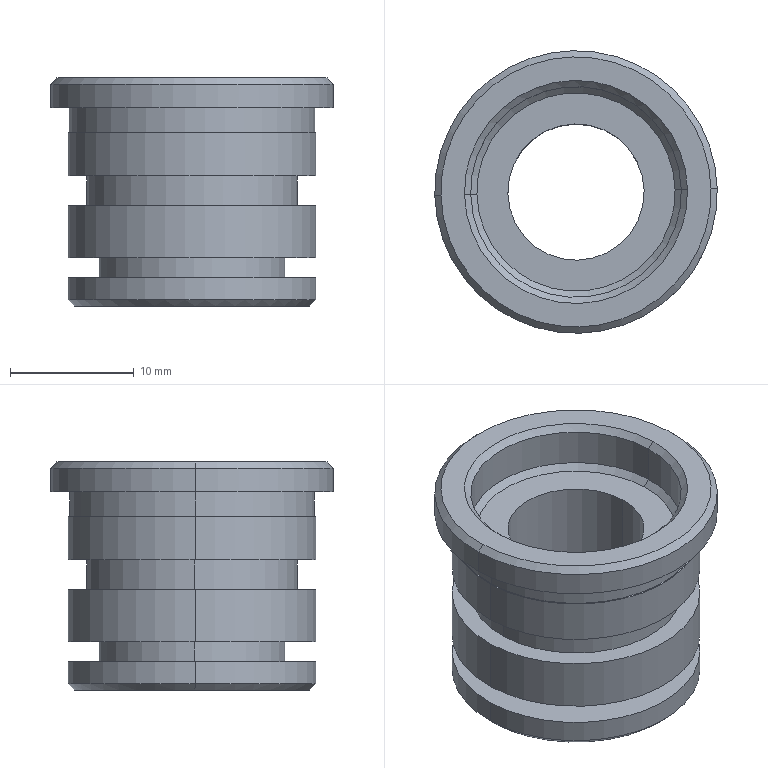Part | SolidWorks | features BaseBody 1 | 1 solid | 37 faces | box 22.8 x 22.8 x 18.4 mm | volume 3267 mm3 | cylinder 18 | cone 10 | plane 9 | commonest cylinder face diameters 20 x6 17 x4 11 x2 15 x2 19.8 x2 22.8 x2
STEP:
#1=CARTESIAN_POINT('',(394.496,102.788,49.));
#2=VERTEX_POINT('',#1);
#3=CARTESIAN_POINT('',(371.704,102.212,49.));
#4=VERTEX_POINT('',#3);
#5=CARTESIAN_POINT('',(383.1,102.5,49.));
#6=DIRECTION('',(0.,0.,-1.));
#7=DIRECTION('',(0.9997,0.02523,0.));
#8=AXIS2_PLACEMENT_3D('',#5,#6,#7);
#9=CIRCLE('',#8,11.4);
#10=EDGE_CURVE('',#2,#4,#9,.T.);
#11=ORIENTED_EDGE('',*,*,#10,.T.);
#12=CARTESIAN_POINT('',(371.704,102.212,47.1));
#13=VERTEX_POINT('',#12);
#14=CARTESIAN_POINT('',(371.704,102.212,25.779));
#15=DIRECTION('',(0.,0.,-1.));
#16=VECTOR('',#15,1000.);
#17=LINE('',#14,#16);
#18=EDGE_CURVE('',#4,#13,#17,.T.);
#19=ORIENTED_EDGE('',*,*,#18,.T.);
#20=CARTESIAN_POINT('',(394.496,102.788,47.1));
#21=VERTEX_POINT('',#20);
#22=CARTESIAN_POINT('',(383.1,102.5,47.1));
#23=DIRECTION('',(0.,0.,-1.));
#24=DIRECTION('',(0.9997,0.02523,0.));
#25=AXIS2_PLACEMENT_3D('',#22,#23,#24);
#26=CIRCLE('',#25,11.4);
#27=EDGE_CURVE('',#21,#13,#26,.T.);
#28=ORIENTED_EDGE('',*,*,#27,.F.);
#29=CARTESIAN_POINT('',(394.496,102.788,25.779));
#30=DIRECTION('',(0.,0.,-1.));
#31=VECTOR('',#30,1000.);
#32=LINE('',#29,#31);
#33=EDGE_CURVE('',#2,#21,#32,.T.);
#34=ORIENTED_EDGE('',*,*,#33,.F.);
#35=EDGE_LOOP('',(#11,#19,#28,#34));
#36=FACE_OUTER_BOUND('',#35,.T.);
#37=CARTESIAN_POINT('',(383.1,102.5,25.779));
#38=DIRECTION('',(0.,0.,-1.));
#39=DIRECTION('',(0.9997,0.02523,0.));
#40=AXIS2_PLACEMENT_3D('',#37,#38,#39);
#41=CYLINDRICAL_SURFACE('',#40,11.4);
#42=ADVANCED_FACE('',(#36),#41,.T.);
#43=CARTESIAN_POINT('',(393.997,102.775,49.5));
#44=VERTEX_POINT('',#43);
#45=CARTESIAN_POINT('',(372.203,102.225,49.5));
#46=VERTEX_POINT('',#45);
#47=CARTESIAN_POINT('',(383.1,102.5,49.5));
#48=DIRECTION('',(0.,0.,-1.));
#49=DIRECTION('',(0.9997,0.02523,0.));
#50=AXIS2_PLACEMENT_3D('',#47,#48,#49);
#51=CIRCLE('',#50,10.9);
#52=EDGE_CURVE('',#44,#46,#51,.T.);
#53=ORIENTED_EDGE('',*,*,#52,.T.);
#54=CARTESIAN_POINT('',(371.704,102.212,49.));
#55=DIRECTION('',(-0.7069,-0.01784,-0.7071));
#56=VECTOR('',#55,1000.);
#57=LINE('',#54,#56);
#58=EDGE_CURVE('',#46,#4,#57,.T.);
#59=ORIENTED_EDGE('',*,*,#58,.T.);
#60=ORIENTED_EDGE('',*,*,#10,.F.);
#61=CARTESIAN_POINT('',(394.496,102.788,49.));
#62=DIRECTION('',(0.7069,0.01784,-0.7071));
#63=VECTOR('',#62,1000.);
#64=LINE('',#61,#63);
#65=EDGE_CURVE('',#44,#2,#64,.T.);
#66=ORIENTED_EDGE('',*,*,#65,.F.);
#67=EDGE_LOOP('',(#53,#59,#60,#66));
#68=FACE_OUTER_BOUND('',#67,.T.);
#69=CARTESIAN_POINT('',(383.1,102.5,49.));
#70=DIRECTION('',(0.,0.,-1.));
#71=DIRECTION('',(0.9997,0.02523,0.));
#72=AXIS2_PLACEMENT_3D('',#69,#70,#71);
#73=CONICAL_SURFACE('',#72,11.4,0.7854);
#74=ADVANCED_FACE('',(#68),#73,.T.);
#75=CARTESIAN_POINT('',(374.603,102.286,49.));
#76=VERTEX_POINT('',#75);
#77=CARTESIAN_POINT('',(391.597,102.714,49.));
#78=VERTEX_POINT('',#77);
#79=CARTESIAN_POINT('',(383.1,102.5,49.));
#80=DIRECTION('',(0.,0.,-1.));
#81=DIRECTION('',(0.9997,0.02523,0.));
#82=AXIS2_PLACEMENT_3D('',#79,#80,#81);
#83=CIRCLE('',#82,8.5);
#84=EDGE_CURVE('',#76,#78,#83,.T.);
#85=ORIENTED_EDGE('',*,*,#84,.T.);
#86=CARTESIAN_POINT('',(392.097,102.727,49.5));
#87=VERTEX_POINT('',#86);
#88=CARTESIAN_POINT('',(392.097,102.727,49.5));
#89=DIRECTION('',(0.7069,0.01784,0.7071));
#90=VECTOR('',#89,1000.);
#91=LINE('',#88,#90);
#92=EDGE_CURVE('',#78,#87,#91,.T.);
#93=ORIENTED_EDGE('',*,*,#92,.T.);
#94=CARTESIAN_POINT('',(374.103,102.273,49.5));
#95=VERTEX_POINT('',#94);
#96=CARTESIAN_POINT('',(383.1,102.5,49.5));
#97=DIRECTION('',(0.,0.,-1.));
#98=DIRECTION('',(0.9997,0.02523,0.));
#99=AXIS2_PLACEMENT_3D('',#96,#97,#98);
#100=CIRCLE('',#99,9.);
#101=EDGE_CURVE('',#95,#87,#100,.T.);
#102=ORIENTED_EDGE('',*,*,#101,.F.);
#103=CARTESIAN_POINT('',(374.103,102.273,49.5));
#104=DIRECTION('',(-0.7069,-0.01784,0.7071));
#105=VECTOR('',#104,1000.);
#106=LINE('',#103,#105);
#107=EDGE_CURVE('',#76,#95,#106,.T.);
#108=ORIENTED_EDGE('',*,*,#107,.F.);
#109=EDGE_LOOP('',(#85,#93,#102,#108));
#110=FACE_OUTER_BOUND('',#109,.T.);
#111=CARTESIAN_POINT('',(383.1,102.5,49.5));
#112=DIRECTION('',(0.,0.,1.));
#113=DIRECTION('',(-0.9997,-0.02523,0.));
#114=AXIS2_PLACEMENT_3D('',#111,#112,#113);
#115=CONICAL_SURFACE('',#114,9.,0.7854);
#116=ADVANCED_FACE('',(#110),#115,.F.);
#117=ORIENTED_EDGE('',*,*,#84,.F.);
#118=CARTESIAN_POINT('',(374.603,102.286,46.));
#119=VERTEX_POINT('',#118);
#120=CARTESIAN_POINT('',(374.603,102.286,25.779));
#121=DIRECTION('',(0.,0.,-1.));
#122=VECTOR('',#121,1000.);
#123=LINE('',#120,#122);
#124=EDGE_CURVE('',#76,#119,#123,.T.);
#125=ORIENTED_EDGE('',*,*,#124,.T.);
#126=CARTESIAN_POINT('',(391.597,102.714,46.));
#127=VERTEX_POINT('',#126);
#128=CARTESIAN_POINT('',(383.1,102.5,46.));
#129=DIRECTION('',(0.,0.,-1.));
#130=DIRECTION('',(0.9997,0.02523,0.));
#131=AXIS2_PLACEMENT_3D('',#128,#129,#130);
#132=CIRCLE('',#131,8.5);
#133=EDGE_CURVE('',#119,#127,#132,.T.);
#134=ORIENTED_EDGE('',*,*,#133,.T.);
#135=CARTESIAN_POINT('',(391.597,102.714,25.779));
#136=DIRECTION('',(0.,0.,-1.));
#137=VECTOR('',#136,1000.);
#138=LINE('',#135,#137);
#139=EDGE_CURVE('',#78,#127,#138,.T.);
#140=ORIENTED_EDGE('',*,*,#139,.F.);
#141=EDGE_LOOP('',(#117,#125,#134,#140));
#142=FACE_OUTER_BOUND('',#141,.T.);
#143=CARTESIAN_POINT('',(383.1,102.5,25.779));
#144=DIRECTION('',(0.,0.,-1.));
#145=DIRECTION('',(0.9997,0.02523,0.));
#146=AXIS2_PLACEMENT_3D('',#143,#144,#145);
#147=CYLINDRICAL_SURFACE('',#146,8.5);
#148=ADVANCED_FACE('',(#142),#147,.F.);
#149=CARTESIAN_POINT('',(375.103,102.298,45.5));
#150=VERTEX_POINT('',#149);
#151=CARTESIAN_POINT('',(391.097,102.702,45.5));
#152=VERTEX_POINT('',#151);
#153=CARTESIAN_POINT('',(383.1,102.5,45.5));
#154=DIRECTION('',(0.,0.,-1.));
#155=DIRECTION('',(0.9997,0.02523,0.));
#156=AXIS2_PLACEMENT_3D('',#153,#154,#155);
#157=CIRCLE('',#156,8.);
#158=EDGE_CURVE('',#150,#152,#157,.T.);
#159=ORIENTED_EDGE('',*,*,#158,.T.);
#160=CARTESIAN_POINT('',(391.597,102.714,46.));
#161=DIRECTION('',(0.7069,0.01784,0.7071));
#162=VECTOR('',#161,1000.);
#163=LINE('',#160,#162);
#164=EDGE_CURVE('',#152,#127,#163,.T.);
#165=ORIENTED_EDGE('',*,*,#164,.T.);
#166=ORIENTED_EDGE('',*,*,#133,.F.);
#167=CARTESIAN_POINT('',(374.603,102.286,46.));
#168=DIRECTION('',(-0.7069,-0.01784,0.7071));
#169=VECTOR('',#168,1000.);
#170=LINE('',#167,#169);
#171=EDGE_CURVE('',#150,#119,#170,.T.);
#172=ORIENTED_EDGE('',*,*,#171,.F.);
#173=EDGE_LOOP('',(#159,#165,#166,#172));
#174=FACE_OUTER_BOUND('',#173,.T.);
#175=CARTESIAN_POINT('',(383.1,102.5,46.));
#176=DIRECTION('',(0.,0.,1.));
#177=DIRECTION('',(-0.9997,-0.02523,0.));
#178=AXIS2_PLACEMENT_3D('',#175,#176,#177);
#179=CONICAL_SURFACE('',#178,8.5,0.7854);
#180=ADVANCED_FACE('',(#174),#179,.F.);
#181=CARTESIAN_POINT('',(377.602,102.361,45.5));
#182=VERTEX_POINT('',#181);
#183=CARTESIAN_POINT('',(388.598,102.639,45.5));
#184=VERTEX_POINT('',#183);
#185=CARTESIAN_POINT('',(383.1,102.5,45.5));
#186=DIRECTION('',(0.,0.,-1.));
#187=DIRECTION('',(0.9997,0.02523,0.));
#188=AXIS2_PLACEMENT_3D('',#185,#186,#187);
#189=CIRCLE('',#188,5.5);
#190=EDGE_CURVE('',#182,#184,#189,.T.);
#191=ORIENTED_EDGE('',*,*,#190,.F.);
#192=CARTESIAN_POINT('',(377.602,102.361,31.6));
#193=VERTEX_POINT('',#192);
#194=CARTESIAN_POINT('',(377.602,102.361,25.779));
#195=DIRECTION('',(0.,0.,-1.));
#196=VECTOR('',#195,1000.);
#197=LINE('',#194,#196);
#198=EDGE_CURVE('',#182,#193,#197,.T.);
#199=ORIENTED_EDGE('',*,*,#198,.T.);
#200=CARTESIAN_POINT('',(388.598,102.639,31.6));
#201=VERTEX_POINT('',#200);
#202=CARTESIAN_POINT('',(383.1,102.5,31.6));
#203=DIRECTION('',(0.,0.,-1.));
#204=DIRECTION('',(0.9997,0.02523,0.));
#205=AXIS2_PLACEMENT_3D('',#202,#203,#204);
#206=CIRCLE('',#205,5.5);
#207=EDGE_CURVE('',#193,#201,#206,.T.);
#208=ORIENTED_EDGE('',*,*,#207,.T.);
#209=CARTESIAN_POINT('',(388.598,102.639,25.779));
#210=DIRECTION('',(0.,0.,-1.));
#211=VECTOR('',#210,1000.);
#212=LINE('',#209,#211);
#213=EDGE_CURVE('',#184,#201,#212,.T.);
#214=ORIENTED_EDGE('',*,*,#213,.F.);
#215=EDGE_LOOP('',(#191,#199,#208,#214));
#216=FACE_OUTER_BOUND('',#215,.T.);
#217=CARTESIAN_POINT('',(383.1,102.5,25.779));
#218=DIRECTION('',(0.,0.,-1.));
#219=DIRECTION('',(0.9997,0.02523,0.));
#220=AXIS2_PLACEMENT_3D('',#217,#218,#219);
#221=CYLINDRICAL_SURFACE('',#220,5.5);
#222=ADVANCED_FACE('',(#216),#221,.F.);
#223=ORIENTED_EDGE('',*,*,#207,.F.);
#224=CARTESIAN_POINT('',(377.102,102.349,31.1));
#225=VERTEX_POINT('',#224);
#226=CARTESIAN_POINT('',(377.602,102.361,31.6));
#227=DIRECTION('',(-0.7069,-0.01784,-0.7071));
#228=VECTOR('',#227,1000.);
#229=LINE('',#226,#228);
#230=EDGE_CURVE('',#193,#225,#229,.T.);
#231=ORIENTED_EDGE('',*,*,#230,.T.);
#232=CARTESIAN_POINT('',(389.098,102.651,31.1));
#233=VERTEX_POINT('',#232);
#234=CARTESIAN_POINT('',(383.1,102.5,31.1));
#235=DIRECTION('',(0.,0.,-1.));
#236=DIRECTION('',(0.9997,0.02523,0.));
#237=AXIS2_PLACEMENT_3D('',#234,#235,#236);
#238=CIRCLE('',#237,6.);
#239=EDGE_CURVE('',#225,#233,#238,.T.);
#240=ORIENTED_EDGE('',*,*,#239,.T.);
#241=CARTESIAN_POINT('',(388.598,102.639,31.6));
#242=DIRECTION('',(0.7069,0.01784,-0.7071));
#243=VECTOR('',#242,1000.);
#244=LINE('',#241,#243);
#245=EDGE_CURVE('',#201,#233,#244,.T.);
#246=ORIENTED_EDGE('',*,*,#245,.F.);
#247=EDGE_LOOP('',(#223,#231,#240,#246));
#248=FACE_OUTER_BOUND('',#247,.T.);
#249=CARTESIAN_POINT('',(383.1,102.5,31.6));
#250=DIRECTION('',(0.,0.,-1.));
#251=DIRECTION('',(0.9997,0.02523,0.));
#252=AXIS2_PLACEMENT_3D('',#249,#250,#251);
#253=CONICAL_SURFACE('',#252,5.5,0.7854);
#254=ADVANCED_FACE('',(#248),#253,.F.);
#255=CARTESIAN_POINT('',(392.597,102.74,31.1));
#256=VERTEX_POINT('',#255);
#257=CARTESIAN_POINT('',(373.603,102.26,31.1));
#258=VERTEX_POINT('',#257);
#259=CARTESIAN_POINT('',(383.1,102.5,31.1));
#260=DIRECTION('',(0.,0.,-1.));
#261=DIRECTION('',(0.9997,0.02523,0.));
#262=AXIS2_PLACEMENT_3D('',#259,#260,#261);
#263=CIRCLE('',#262,9.5);
#264=EDGE_CURVE('',#256,#258,#263,.T.);
#265=ORIENTED_EDGE('',*,*,#264,.F.);
#266=CARTESIAN_POINT('',(393.097,102.752,31.6));
#267=VERTEX_POINT('',#266);
#268=CARTESIAN_POINT('',(392.597,102.74,31.1));
#269=DIRECTION('',(0.7069,0.01784,0.7071));
#270=VECTOR('',#269,1000.);
#271=LINE('',#268,#270);
#272=EDGE_CURVE('',#256,#267,#271,.T.);
#273=ORIENTED_EDGE('',*,*,#272,.T.);
#274=CARTESIAN_POINT('',(373.103,102.248,31.6));
#275=VERTEX_POINT('',#274);
#276=CARTESIAN_POINT('',(383.1,102.5,31.6));
#277=DIRECTION('',(0.,0.,-1.));
#278=DIRECTION('',(0.9997,0.02523,0.));
#279=AXIS2_PLACEMENT_3D('',#276,#277,#278);
#280=CIRCLE('',#279,10.);
#281=EDGE_CURVE('',#267,#275,#280,.T.);
#282=ORIENTED_EDGE('',*,*,#281,.T.);
#283=CARTESIAN_POINT('',(373.603,102.26,31.1));
#284=DIRECTION('',(-0.7069,-0.01784,0.7071));
#285=VECTOR('',#284,1000.);
#286=LINE('',#283,#285);
#287=EDGE_CURVE('',#258,#275,#286,.T.);
#288=ORIENTED_EDGE('',*,*,#287,.F.);
#289=EDGE_LOOP('',(#265,#273,#282,#288));
#290=FACE_OUTER_BOUND('',#289,.T.);
#291=CARTESIAN_POINT('',(383.1,102.5,31.1));
#292=DIRECTION('',(0.,0.,1.));
#293=DIRECTION('',(-0.9997,-0.02523,0.));
#294=AXIS2_PLACEMENT_3D('',#291,#292,#293);
#295=CONICAL_SURFACE('',#294,9.5,0.7854);
#296=ADVANCED_FACE('',(#290),#295,.T.);
#297=CARTESIAN_POINT('',(393.097,102.752,33.4));
#298=VERTEX_POINT('',#297);
#299=CARTESIAN_POINT('',(373.103,102.248,33.4));
#300=VERTEX_POINT('',#299);
#301=CARTESIAN_POINT('',(383.1,102.5,33.4));
#302=DIRECTION('',(0.,0.,-1.));
#303=DIRECTION('',(0.9997,0.02523,0.));
#304=AXIS2_PLACEMENT_3D('',#301,#302,#303);
#305=CIRCLE('',#304,10.);
#306=EDGE_CURVE('',#298,#300,#305,.T.);
#307=ORIENTED_EDGE('',*,*,#306,.T.);
#308=CARTESIAN_POINT('',(373.103,102.248,25.779));
#309=DIRECTION('',(0.,0.,-1.));
#310=VECTOR('',#309,1000.);
#311=LINE('',#308,#310);
#312=EDGE_CURVE('',#300,#275,#311,.T.);
#313=ORIENTED_EDGE('',*,*,#312,.T.);
#314=ORIENTED_EDGE('',*,*,#281,.F.);
#315=CARTESIAN_POINT('',(393.097,102.752,25.779));
#316=DIRECTION('',(0.,0.,-1.));
#317=VECTOR('',#316,1000.);
#318=LINE('',#315,#317);
#319=EDGE_CURVE('',#298,#267,#318,.T.);
#320=ORIENTED_EDGE('',*,*,#319,.F.);
#321=EDGE_LOOP('',(#307,#313,#314,#320));
#322=FACE_OUTER_BOUND('',#321,.T.);
#323=CARTESIAN_POINT('',(383.1,102.5,25.779));
#324=DIRECTION('',(0.,0.,-1.));
#325=DIRECTION('',(0.9997,0.02523,0.));
#326=AXIS2_PLACEMENT_3D('',#323,#324,#325);
#327=CYLINDRICAL_SURFACE('',#326,10.);
#328=ADVANCED_FACE('',(#322),#327,.T.);
#329=CARTESIAN_POINT('',(390.598,102.689,35.));
#330=VERTEX_POINT('',#329);
#331=CARTESIAN_POINT('',(375.602,102.311,35.));
#332=VERTEX_POINT('',#331);
#333=CARTESIAN_POINT('',(383.1,102.5,35.));
#334=DIRECTION('',(0.,0.,-1.));
#335=DIRECTION('',(0.9997,0.02523,0.));
#336=AXIS2_PLACEMENT_3D('',#333,#334,#335);
#337=CIRCLE('',#336,7.5);
#338=EDGE_CURVE('',#330,#332,#337,.T.);
#339=ORIENTED_EDGE('',*,*,#338,.T.);
#340=CARTESIAN_POINT('',(375.602,102.311,33.4));
#341=VERTEX_POINT('',#340);
#342=CARTESIAN_POINT('',(375.602,102.311,25.779));
#343=DIRECTION('',(0.,0.,-1.));
#344=VECTOR('',#343,1000.);
#345=LINE('',#342,#344);
#346=EDGE_CURVE('',#332,#341,#345,.T.);
#347=ORIENTED_EDGE('',*,*,#346,.T.);
#348=CARTESIAN_POINT('',(390.598,102.689,33.4));
#349=VERTEX_POINT('',#348);
#350=CARTESIAN_POINT('',(383.1,102.5,33.4));
#351=DIRECTION('',(0.,0.,-1.));
#352=DIRECTION('',(0.9997,0.02523,0.));
#353=AXIS2_PLACEMENT_3D('',#350,#351,#352);
#354=CIRCLE('',#353,7.5);
#355=EDGE_CURVE('',#349,#341,#354,.T.);
#356=ORIENTED_EDGE('',*,*,#355,.F.);
#357=CARTESIAN_POINT('',(390.598,102.689,25.779));
#358=DIRECTION('',(0.,0.,-1.));
#359=VECTOR('',#358,1000.);
#360=LINE('',#357,#359);
#361=EDGE_CURVE('',#330,#349,#360,.T.);
#362=ORIENTED_EDGE('',*,*,#361,.F.);
#363=EDGE_LOOP('',(#339,#347,#356,#362));
#364=FACE_OUTER_BOUND('',#363,.T.);
#365=CARTESIAN_POINT('',(383.1,102.5,25.779));
#366=DIRECTION('',(0.,0.,-1.));
#367=DIRECTION('',(0.9997,0.02523,0.));
#368=AXIS2_PLACEMENT_3D('',#365,#366,#367);
#369=CYLINDRICAL_SURFACE('',#368,7.5);
#370=ADVANCED_FACE('',(#364),#369,.T.);
#371=CARTESIAN_POINT('',(393.097,102.752,39.2));
#372=VERTEX_POINT('',#371);
#373=CARTESIAN_POINT('',(373.103,102.248,39.2));
#374=VERTEX_POINT('',#373);
#375=CARTESIAN_POINT('',(383.1,102.5,39.2));
#376=DIRECTION('',(0.,0.,-1.));
#377=DIRECTION('',(0.9997,0.02523,0.));
#378=AXIS2_PLACEMENT_3D('',#375,#376,#377);
#379=CIRCLE('',#378,10.);
#380=EDGE_CURVE('',#372,#374,#379,.T.);
#381=ORIENTED_EDGE('',*,*,#380,.T.);
#382=CARTESIAN_POINT('',(373.103,102.248,35.));
#383=VERTEX_POINT('',#382);
#384=CARTESIAN_POINT('',(373.103,102.248,25.779));
#385=DIRECTION('',(0.,0.,-1.));
#386=VECTOR('',#385,1000.);
#387=LINE('',#384,#386);
#388=EDGE_CURVE('',#374,#383,#387,.T.);
#389=ORIENTED_EDGE('',*,*,#388,.T.);
#390=CARTESIAN_POINT('',(393.097,102.752,35.));
#391=VERTEX_POINT('',#390);
#392=CARTESIAN_POINT('',(383.1,102.5,35.));
#393=DIRECTION('',(0.,0.,-1.));
#394=DIRECTION('',(0.9997,0.02523,0.));
#395=AXIS2_PLACEMENT_3D('',#392,#393,#394);
#396=CIRCLE('',#395,10.);
#397=EDGE_CURVE('',#391,#383,#396,.T.);
#398=ORIENTED_EDGE('',*,*,#397,.F.);
#399=CARTESIAN_POINT('',(393.097,102.752,25.779));
#400=DIRECTION('',(0.,0.,-1.));
#401=VECTOR('',#400,1000.);
#402=LINE('',#399,#401);
#403=EDGE_CURVE('',#372,#391,#402,.T.);
#404=ORIENTED_EDGE('',*,*,#403,.F.);
#405=EDGE_LOOP('',(#381,#389,#398,#404));
#406=FACE_OUTER_BOUND('',#405,.T.);
#407=CARTESIAN_POINT('',(383.1,102.5,25.779));
#408=DIRECTION('',(0.,0.,-1.));
#409=DIRECTION('',(0.9997,0.02523,0.));
#410=AXIS2_PLACEMENT_3D('',#407,#408,#409);
#411=CYLINDRICAL_SURFACE('',#410,10.);
#412=ADVANCED_FACE('',(#406),#411,.T.);
#413=CARTESIAN_POINT('',(391.597,102.714,41.6));
#414=VERTEX_POINT('',#413);
#415=CARTESIAN_POINT('',(374.603,102.286,41.6));
#416=VERTEX_POINT('',#415);
#417=CARTESIAN_POINT('',(383.1,102.5,41.6));
#418=DIRECTION('',(0.,0.,-1.));
#419=DIRECTION('',(0.9997,0.02523,0.));
#420=AXIS2_PLACEMENT_3D('',#417,#418,#419);
#421=CIRCLE('',#420,8.5);
#422=EDGE_CURVE('',#414,#416,#421,.T.);
#423=ORIENTED_EDGE('',*,*,#422,.T.);
#424=CARTESIAN_POINT('',(374.603,102.286,39.2));
#425=VERTEX_POINT('',#424);
#426=CARTESIAN_POINT('',(374.603,102.286,25.779));
#427=DIRECTION('',(0.,0.,-1.));
#428=VECTOR('',#427,1000.);
#429=LINE('',#426,#428);
#430=EDGE_CURVE('',#416,#425,#429,.T.);
#431=ORIENTED_EDGE('',*,*,#430,.T.);
#432=CARTESIAN_POINT('',(391.597,102.714,39.2));
#433=VERTEX_POINT('',#432);
#434=CARTESIAN_POINT('',(383.1,102.5,39.2));
#435=DIRECTION('',(0.,0.,-1.));
#436=DIRECTION('',(0.9997,0.02523,0.));
#437=AXIS2_PLACEMENT_3D('',#434,#435,#436);
#438=CIRCLE('',#437,8.5);
#439=EDGE_CURVE('',#433,#425,#438,.T.);
#440=ORIENTED_EDGE('',*,*,#439,.F.);
#441=CARTESIAN_POINT('',(391.597,102.714,25.779));
#442=DIRECTION('',(0.,0.,-1.));
#443=VECTOR('',#442,1000.);
#444=LINE('',#441,#443);
#445=EDGE_CURVE('',#414,#433,#444,.T.);
#446=ORIENTED_EDGE('',*,*,#445,.F.);
#447=EDGE_LOOP('',(#423,#431,#440,#446));
#448=FACE_OUTER_BOUND('',#447,.T.);
#449=CARTESIAN_POINT('',(383.1,102.5,25.779));
#450=DIRECTION('',(0.,0.,-1.));
#451=DIRECTION('',(0.9997,0.02523,0.));
#452=AXIS2_PLACEMENT_3D('',#449,#450,#451);
#453=CYLINDRICAL_SURFACE('',#452,8.5);
#454=ADVANCED_FACE('',(#448),#453,.T.);
#455=CARTESIAN_POINT('',(393.097,102.752,45.1));
#456=VERTEX_POINT('',#455);
#457=CARTESIAN_POINT('',(373.103,102.248,45.1));
#458=VERTEX_POINT('',#457);
#459=CARTESIAN_POINT('',(383.1,102.5,45.1));
#460=DIRECTION('',(0.,0.,-1.));
#461=DIRECTION('',(0.9997,0.02523,0.));
#462=AXIS2_PLACEMENT_3D('',#459,#460,#461);
#463=CIRCLE('',#462,10.);
#464=EDGE_CURVE('',#456,#458,#463,.T.);
#465=ORIENTED_EDGE('',*,*,#464,.T.);
#466=CARTESIAN_POINT('',(373.103,102.248,41.6));
#467=VERTEX_POINT('',#466);
#468=CARTESIAN_POINT('',(373.103,102.248,25.779));
#469=DIRECTION('',(0.,0.,-1.));
#470=VECTOR('',#469,1000.);
#471=LINE('',#468,#470);
#472=EDGE_CURVE('',#458,#467,#471,.T.);
#473=ORIENTED_EDGE('',*,*,#472,.T.);
#474=CARTESIAN_POINT('',(393.097,102.752,41.6));
#475=VERTEX_POINT('',#474);
#476=CARTESIAN_POINT('',(383.1,102.5,41.6));
#477=DIRECTION('',(0.,0.,-1.));
#478=DIRECTION('',(0.9997,0.02523,0.));
#479=AXIS2_PLACEMENT_3D('',#476,#477,#478);
#480=CIRCLE('',#479,10.);
#481=EDGE_CURVE('',#475,#467,#480,.T.);
#482=ORIENTED_EDGE('',*,*,#481,.F.);
#483=CARTESIAN_POINT('',(393.097,102.752,25.779));
#484=DIRECTION('',(0.,0.,-1.));
#485=VECTOR('',#484,1000.);
#486=LINE('',#483,#485);
#487=EDGE_CURVE('',#456,#475,#486,.T.);
#488=ORIENTED_EDGE('',*,*,#487,.F.);
#489=EDGE_LOOP('',(#465,#473,#482,#488));
#490=FACE_OUTER_BOUND('',#489,.T.);
#491=CARTESIAN_POINT('',(383.1,102.5,25.779));
#492=DIRECTION('',(0.,0.,-1.));
#493=DIRECTION('',(0.9997,0.02523,0.));
#494=AXIS2_PLACEMENT_3D('',#491,#492,#493);
#495=CYLINDRICAL_SURFACE('',#494,10.);
#496=ADVANCED_FACE('',(#490),#495,.T.);
#497=CARTESIAN_POINT('',(392.997,102.75,47.1));
#498=VERTEX_POINT('',#497);
#499=CARTESIAN_POINT('',(373.203,102.25,47.1));
#500=VERTEX_POINT('',#499);
#501=CARTESIAN_POINT('',(383.1,102.5,47.1));
#502=DIRECTION('',(0.,0.,-1.));
#503=DIRECTION('',(0.9997,0.02523,0.));
#504=AXIS2_PLACEMENT_3D('',#501,#502,#503);
#505=CIRCLE('',#504,9.9);
#506=EDGE_CURVE('',#498,#500,#505,.T.);
#507=ORIENTED_EDGE('',*,*,#506,.T.);
#508=CARTESIAN_POINT('',(373.203,102.25,45.1));
#509=VERTEX_POINT('',#508);
#510=CARTESIAN_POINT('',(373.203,102.25,25.779));
#511=DIRECTION('',(0.,0.,-1.));
#512=VECTOR('',#511,1000.);
#513=LINE('',#510,#512);
#514=EDGE_CURVE('',#500,#509,#513,.T.);
#515=ORIENTED_EDGE('',*,*,#514,.T.);
#516=CARTESIAN_POINT('',(392.997,102.75,45.1));
#517=VERTEX_POINT('',#516);
#518=CARTESIAN_POINT('',(383.1,102.5,45.1));
#519=DIRECTION('',(0.,0.,-1.));
#520=DIRECTION('',(0.9997,0.02523,0.));
#521=AXIS2_PLACEMENT_3D('',#518,#519,#520);
#522=CIRCLE('',#521,9.9);
#523=EDGE_CURVE('',#517,#509,#522,.T.);
#524=ORIENTED_EDGE('',*,*,#523,.F.);
#525=CARTESIAN_POINT('',(392.997,102.75,25.779));
#526=DIRECTION('',(0.,0.,-1.));
#527=VECTOR('',#526,1000.);
#528=LINE('',#525,#527);
#529=EDGE_CURVE('',#498,#517,#528,.T.);
#530=ORIENTED_EDGE('',*,*,#529,.F.);
#531=EDGE_LOOP('',(#507,#515,#524,#530));
#532=FACE_OUTER_BOUND('',#531,.T.);
#533=CARTESIAN_POINT('',(383.1,102.5,25.779));
#534=DIRECTION('',(0.,0.,-1.));
#535=DIRECTION('',(0.9997,0.02523,0.));
#536=AXIS2_PLACEMENT_3D('',#533,#534,#535);
#537=CYLINDRICAL_SURFACE('',#536,9.9);
#538=ADVANCED_FACE('',(#532),#537,.T.);
#539=ORIENTED_EDGE('',*,*,#514,.F.);
#540=CARTESIAN_POINT('',(383.1,102.5,47.1));
#541=DIRECTION('',(0.,0.,-1.));
#542=DIRECTION('',(0.9997,0.02523,0.));
#543=AXIS2_PLACEMENT_3D('',#540,#541,#542);
#544=CIRCLE('',#543,9.9);
#545=EDGE_CURVE('',#500,#498,#544,.T.);
#546=ORIENTED_EDGE('',*,*,#545,.T.);
#547=ORIENTED_EDGE('',*,*,#529,.T.);
#548=CARTESIAN_POINT('',(383.1,102.5,45.1));
#549=DIRECTION('',(0.,0.,-1.));
#550=DIRECTION('',(0.9997,0.02523,0.));
#551=AXIS2_PLACEMENT_3D('',#548,#549,#550);
#552=CIRCLE('',#551,9.9);
#553=EDGE_CURVE('',#509,#517,#552,.T.);
#554=ORIENTED_EDGE('',*,*,#553,.F.);
#555=EDGE_LOOP('',(#539,#546,#547,#554));
#556=FACE_OUTER_BOUND('',#555,.T.);
#557=CARTESIAN_POINT('',(383.1,102.5,25.779));
#558=DIRECTION('',(0.,0.,-1.));
#559=DIRECTION('',(0.9997,0.02523,0.));
#560=AXIS2_PLACEMENT_3D('',#557,#558,#559);
#561=CYLINDRICAL_SURFACE('',#560,9.9);
#562=ADVANCED_FACE('',(#556),#561,.T.);
#563=ORIENTED_EDGE('',*,*,#523,.T.);
#564=ORIENTED_EDGE('',*,*,#553,.T.);
#565=EDGE_LOOP('',(#563,#564));
#566=FACE_BOUND('',#565,.T.);
#567=ORIENTED_EDGE('',*,*,#464,.F.);
#568=CARTESIAN_POINT('',(383.1,102.5,45.1));
#569=DIRECTION('',(0.,0.,-1.));
#570=DIRECTION('',(0.9997,0.02523,0.));
#571=AXIS2_PLACEMENT_3D('',#568,#569,#570);
#572=CIRCLE('',#571,10.);
#573=EDGE_CURVE('',#458,#456,#572,.T.);
#574=ORIENTED_EDGE('',*,*,#573,.F.);
#575=EDGE_LOOP('',(#567,#574));
#576=FACE_OUTER_BOUND('',#575,.T.);
#577=CARTESIAN_POINT('',(383.35,92.603,45.1));
#578=DIRECTION('',(0.,0.,1.));
#579=DIRECTION('',(-0.9997,-0.02523,0.));
#580=AXIS2_PLACEMENT_3D('',#577,#578,#579);
#581=PLANE('',#580);
#582=ADVANCED_FACE('',(#566,#576),#581,.T.);
#583=ORIENTED_EDGE('',*,*,#472,.F.);
#584=ORIENTED_EDGE('',*,*,#573,.T.);
#585=ORIENTED_EDGE('',*,*,#487,.T.);
#586=CARTESIAN_POINT('',(383.1,102.5,41.6));
#587=DIRECTION('',(0.,0.,-1.));
#588=DIRECTION('',(0.9997,0.02523,0.));
#589=AXIS2_PLACEMENT_3D('',#586,#587,#588);
#590=CIRCLE('',#589,10.);
#591=EDGE_CURVE('',#467,#475,#590,.T.);
#592=ORIENTED_EDGE('',*,*,#591,.F.);
#593=EDGE_LOOP('',(#583,#584,#585,#592));
#594=FACE_OUTER_BOUND('',#593,.T.);
#595=CARTESIAN_POINT('',(383.1,102.5,25.779));
#596=DIRECTION('',(0.,0.,-1.));
#597=DIRECTION('',(0.9997,0.02523,0.));
#598=AXIS2_PLACEMENT_3D('',#595,#596,#597);
#599=CYLINDRICAL_SURFACE('',#598,10.);
#600=ADVANCED_FACE('',(#594),#599,.T.);
#601=ORIENTED_EDGE('',*,*,#481,.T.);
#602=ORIENTED_EDGE('',*,*,#591,.T.);
#603=EDGE_LOOP('',(#601,#602));
#604=FACE_OUTER_BOUND('',#603,.T.);
#605=ORIENTED_EDGE('',*,*,#422,.F.);
#606=CARTESIAN_POINT('',(383.1,102.5,41.6));
#607=DIRECTION('',(0.,0.,-1.));
#608=DIRECTION('',(0.9997,0.02523,0.));
#609=AXIS2_PLACEMENT_3D('',#606,#607,#608);
#610=CIRCLE('',#609,8.5);
#611=EDGE_CURVE('',#416,#414,#610,.T.);
#612=ORIENTED_EDGE('',*,*,#611,.F.);
#613=EDGE_LOOP('',(#605,#612));
#614=FACE_BOUND('',#613,.T.);
#615=CARTESIAN_POINT('',(383.314,94.003,41.6));
#616=DIRECTION('',(0.,0.,-1.));
#617=DIRECTION('',(0.9997,0.02523,0.));
#618=AXIS2_PLACEMENT_3D('',#615,#616,#617);
#619=PLANE('',#618);
#620=ADVANCED_FACE('',(#604,#614),#619,.T.);
#621=ORIENTED_EDGE('',*,*,#430,.F.);
#622=ORIENTED_EDGE('',*,*,#611,.T.);
#623=ORIENTED_EDGE('',*,*,#445,.T.);
#624=CARTESIAN_POINT('',(383.1,102.5,39.2));
#625=DIRECTION('',(0.,0.,-1.));
#626=DIRECTION('',(0.9997,0.02523,0.));
#627=AXIS2_PLACEMENT_3D('',#624,#625,#626);
#628=CIRCLE('',#627,8.5);
#629=EDGE_CURVE('',#425,#433,#628,.T.);
#630=ORIENTED_EDGE('',*,*,#629,.F.);
#631=EDGE_LOOP('',(#621,#622,#623,#630));
#632=FACE_OUTER_BOUND('',#631,.T.);
#633=CARTESIAN_POINT('',(383.1,102.5,25.779));
#634=DIRECTION('',(0.,0.,-1.));
#635=DIRECTION('',(0.9997,0.02523,0.));
#636=AXIS2_PLACEMENT_3D('',#633,#634,#635);
#637=CYLINDRICAL_SURFACE('',#636,8.5);
#638=ADVANCED_FACE('',(#632),#637,.T.);
#639=ORIENTED_EDGE('',*,*,#439,.T.);
#640=ORIENTED_EDGE('',*,*,#629,.T.);
#641=EDGE_LOOP('',(#639,#640));
#642=FACE_BOUND('',#641,.T.);
#643=ORIENTED_EDGE('',*,*,#380,.F.);
#644=CARTESIAN_POINT('',(383.1,102.5,39.2));
#645=DIRECTION('',(0.,0.,-1.));
#646=DIRECTION('',(0.9997,0.02523,0.));
#647=AXIS2_PLACEMENT_3D('',#644,#645,#646);
#648=CIRCLE('',#647,10.);
#649=EDGE_CURVE('',#374,#372,#648,.T.);
#650=ORIENTED_EDGE('',*,*,#649,.F.);
#651=EDGE_LOOP('',(#643,#650));
#652=FACE_OUTER_BOUND('',#651,.T.);
#653=CARTESIAN_POINT('',(383.314,94.003,39.2));
#654=DIRECTION('',(0.,0.,1.));
#655=DIRECTION('',(-0.9997,-0.02523,0.));
#656=AXIS2_PLACEMENT_3D('',#653,#654,#655);
#657=PLANE('',#656);
#658=ADVANCED_FACE('',(#642,#652),#657,.T.);
#659=ORIENTED_EDGE('',*,*,#388,.F.);
#660=ORIENTED_EDGE('',*,*,#649,.T.);
#661=ORIENTED_EDGE('',*,*,#403,.T.);
#662=CARTESIAN_POINT('',(383.1,102.5,35.));
#663=DIRECTION('',(0.,0.,-1.));
#664=DIRECTION('',(0.9997,0.02523,0.));
#665=AXIS2_PLACEMENT_3D('',#662,#663,#664);
#666=CIRCLE('',#665,10.);
#667=EDGE_CURVE('',#383,#391,#666,.T.);
#668=ORIENTED_EDGE('',*,*,#667,.F.);
#669=EDGE_LOOP('',(#659,#660,#661,#668));
#670=FACE_OUTER_BOUND('',#669,.T.);
#671=CARTESIAN_POINT('',(383.1,102.5,25.779));
#672=DIRECTION('',(0.,0.,-1.));
#673=DIRECTION('',(0.9997,0.02523,0.));
#674=AXIS2_PLACEMENT_3D('',#671,#672,#673);
#675=CYLINDRICAL_SURFACE('',#674,10.);
#676=ADVANCED_FACE('',(#670),#675,.T.);
#677=ORIENTED_EDGE('',*,*,#397,.T.);
#678=ORIENTED_EDGE('',*,*,#667,.T.);
#679=EDGE_LOOP('',(#677,#678));
#680=FACE_OUTER_BOUND('',#679,.T.);
#681=ORIENTED_EDGE('',*,*,#338,.F.);
#682=CARTESIAN_POINT('',(383.1,102.5,35.));
#683=DIRECTION('',(0.,0.,-1.));
#684=DIRECTION('',(0.9997,0.02523,0.));
#685=AXIS2_PLACEMENT_3D('',#682,#683,#684);
#686=CIRCLE('',#685,7.5);
#687=EDGE_CURVE('',#332,#330,#686,.T.);
#688=ORIENTED_EDGE('',*,*,#687,.F.);
#689=EDGE_LOOP('',(#681,#688));
#690=FACE_BOUND('',#689,.T.);
#691=CARTESIAN_POINT('',(383.289,95.002,35.));
#692=DIRECTION('',(0.,0.,-1.));
#693=DIRECTION('',(0.9997,0.02523,0.));
#694=AXIS2_PLACEMENT_3D('',#691,#692,#693);
#695=PLANE('',#694);
#696=ADVANCED_FACE('',(#680,#690),#695,.T.);
#697=ORIENTED_EDGE('',*,*,#346,.F.);
#698=ORIENTED_EDGE('',*,*,#687,.T.);
#699=ORIENTED_EDGE('',*,*,#361,.T.);
#700=CARTESIAN_POINT('',(383.1,102.5,33.4));
#701=DIRECTION('',(0.,0.,-1.));
#702=DIRECTION('',(0.9997,0.02523,0.));
#703=AXIS2_PLACEMENT_3D('',#700,#701,#702);
#704=CIRCLE('',#703,7.5);
#705=EDGE_CURVE('',#341,#349,#704,.T.);
#706=ORIENTED_EDGE('',*,*,#705,.F.);
#707=EDGE_LOOP('',(#697,#698,#699,#706));
#708=FACE_OUTER_BOUND('',#707,.T.);
#709=CARTESIAN_POINT('',(383.1,102.5,25.779));
#710=DIRECTION('',(0.,0.,-1.));
#711=DIRECTION('',(0.9997,0.02523,0.));
#712=AXIS2_PLACEMENT_3D('',#709,#710,#711);
#713=CYLINDRICAL_SURFACE('',#712,7.5);
#714=ADVANCED_FACE('',(#708),#713,.T.);
#715=ORIENTED_EDGE('',*,*,#355,.T.);
#716=ORIENTED_EDGE('',*,*,#705,.T.);
#717=EDGE_LOOP('',(#715,#716));
#718=FACE_BOUND('',#717,.T.);
#719=ORIENTED_EDGE('',*,*,#306,.F.);
#720=CARTESIAN_POINT('',(383.1,102.5,33.4));
#721=DIRECTION('',(0.,0.,-1.));
#722=DIRECTION('',(0.9997,0.02523,0.));
#723=AXIS2_PLACEMENT_3D('',#720,#721,#722);
#724=CIRCLE('',#723,10.);
#725=EDGE_CURVE('',#300,#298,#724,.T.);
#726=ORIENTED_EDGE('',*,*,#725,.F.);
#727=EDGE_LOOP('',(#719,#726));
#728=FACE_OUTER_BOUND('',#727,.T.);
#729=CARTESIAN_POINT('',(383.289,95.002,33.4));
#730=DIRECTION('',(0.,0.,1.));
#731=DIRECTION('',(-0.9997,-0.02523,0.));
#732=AXIS2_PLACEMENT_3D('',#729,#730,#731);
#733=PLANE('',#732);
#734=ADVANCED_FACE('',(#718,#728),#733,.T.);
#735=ORIENTED_EDGE('',*,*,#312,.F.);
#736=ORIENTED_EDGE('',*,*,#725,.T.);
#737=ORIENTED_EDGE('',*,*,#319,.T.);
#738=CARTESIAN_POINT('',(383.1,102.5,31.6));
#739=DIRECTION('',(0.,0.,-1.));
#740=DIRECTION('',(0.9997,0.02523,0.));
#741=AXIS2_PLACEMENT_3D('',#738,#739,#740);
#742=CIRCLE('',#741,10.);
#743=EDGE_CURVE('',#275,#267,#742,.T.);
#744=ORIENTED_EDGE('',*,*,#743,.F.);
#745=EDGE_LOOP('',(#735,#736,#737,#744));
#746=FACE_OUTER_BOUND('',#745,.T.);
#747=CARTESIAN_POINT('',(383.1,102.5,25.779));
#748=DIRECTION('',(0.,0.,-1.));
#749=DIRECTION('',(0.9997,0.02523,0.));
#750=AXIS2_PLACEMENT_3D('',#747,#748,#749);
#751=CYLINDRICAL_SURFACE('',#750,10.);
#752=ADVANCED_FACE('',(#746),#751,.T.);
#753=ORIENTED_EDGE('',*,*,#272,.F.);
#754=CARTESIAN_POINT('',(383.1,102.5,31.1));
#755=DIRECTION('',(0.,0.,-1.));
#756=DIRECTION('',(0.9997,0.02523,0.));
#757=AXIS2_PLACEMENT_3D('',#754,#755,#756);
#758=CIRCLE('',#757,9.5);
#759=EDGE_CURVE('',#258,#256,#758,.T.);
#760=ORIENTED_EDGE('',*,*,#759,.F.);
#761=ORIENTED_EDGE('',*,*,#287,.T.);
#762=ORIENTED_EDGE('',*,*,#743,.T.);
#763=EDGE_LOOP('',(#753,#760,#761,#762));
#764=FACE_OUTER_BOUND('',#763,.T.);
#765=CARTESIAN_POINT('',(383.1,102.5,31.1));
#766=DIRECTION('',(0.,0.,1.));
#767=DIRECTION('',(-0.9997,-0.02523,0.));
#768=AXIS2_PLACEMENT_3D('',#765,#766,#767);
#769=CONICAL_SURFACE('',#768,9.5,0.7854);
#770=ADVANCED_FACE('',(#764),#769,.T.);
#771=ORIENTED_EDGE('',*,*,#759,.T.);
#772=ORIENTED_EDGE('',*,*,#264,.T.);
#773=EDGE_LOOP('',(#771,#772));
#774=FACE_OUTER_BOUND('',#773,.T.);
#775=CARTESIAN_POINT('',(383.1,102.5,31.1));
#776=DIRECTION('',(0.,0.,-1.));
#777=DIRECTION('',(0.9997,0.02523,0.));
#778=AXIS2_PLACEMENT_3D('',#775,#776,#777);
#779=CIRCLE('',#778,6.);
#780=EDGE_CURVE('',#233,#225,#779,.T.);
#781=ORIENTED_EDGE('',*,*,#780,.F.);
#782=ORIENTED_EDGE('',*,*,#239,.F.);
#783=EDGE_LOOP('',(#781,#782));
#784=FACE_BOUND('',#783,.T.);
#785=CARTESIAN_POINT('',(383.251,96.502,31.1));
#786=DIRECTION('',(0.,0.,-1.));
#787=DIRECTION('',(0.9997,0.02523,0.));
#788=AXIS2_PLACEMENT_3D('',#785,#786,#787);
#789=PLANE('',#788);
#790=ADVANCED_FACE('',(#774,#784),#789,.T.);
#791=ORIENTED_EDGE('',*,*,#230,.F.);
#792=CARTESIAN_POINT('',(383.1,102.5,31.6));
#793=DIRECTION('',(0.,0.,-1.));
#794=DIRECTION('',(0.9997,0.02523,0.));
#795=AXIS2_PLACEMENT_3D('',#792,#793,#794);
#796=CIRCLE('',#795,5.5);
#797=EDGE_CURVE('',#201,#193,#796,.T.);
#798=ORIENTED_EDGE('',*,*,#797,.F.);
#799=ORIENTED_EDGE('',*,*,#245,.T.);
#800=ORIENTED_EDGE('',*,*,#780,.T.);
#801=EDGE_LOOP('',(#791,#798,#799,#800));
#802=FACE_OUTER_BOUND('',#801,.T.);
#803=CARTESIAN_POINT('',(383.1,102.5,31.6));
#804=DIRECTION('',(0.,0.,-1.));
#805=DIRECTION('',(0.9997,0.02523,0.));
#806=AXIS2_PLACEMENT_3D('',#803,#804,#805);
#807=CONICAL_SURFACE('',#806,5.5,0.7854);
#808=ADVANCED_FACE('',(#802),#807,.F.);
#809=ORIENTED_EDGE('',*,*,#198,.F.);
#810=CARTESIAN_POINT('',(383.1,102.5,45.5));
#811=DIRECTION('',(0.,0.,-1.));
#812=DIRECTION('',(0.9997,0.02523,0.));
#813=AXIS2_PLACEMENT_3D('',#810,#811,#812);
#814=CIRCLE('',#813,5.5);
#815=EDGE_CURVE('',#184,#182,#814,.T.);
#816=ORIENTED_EDGE('',*,*,#815,.F.);
#817=ORIENTED_EDGE('',*,*,#213,.T.);
#818=ORIENTED_EDGE('',*,*,#797,.T.);
#819=EDGE_LOOP('',(#809,#816,#817,#818));
#820=FACE_OUTER_BOUND('',#819,.T.);
#821=CARTESIAN_POINT('',(383.1,102.5,25.779));
#822=DIRECTION('',(0.,0.,-1.));
#823=DIRECTION('',(0.9997,0.02523,0.));
#824=AXIS2_PLACEMENT_3D('',#821,#822,#823);
#825=CYLINDRICAL_SURFACE('',#824,5.5);
#826=ADVANCED_FACE('',(#820),#825,.F.);
#827=ORIENTED_EDGE('',*,*,#815,.T.);
#828=ORIENTED_EDGE('',*,*,#190,.T.);
#829=EDGE_LOOP('',(#827,#828));
#830=FACE_BOUND('',#829,.T.);
#831=ORIENTED_EDGE('',*,*,#158,.F.);
#832=CARTESIAN_POINT('',(383.1,102.5,45.5));
#833=DIRECTION('',(0.,0.,-1.));
#834=DIRECTION('',(0.9997,0.02523,0.));
#835=AXIS2_PLACEMENT_3D('',#832,#833,#834);
#836=CIRCLE('',#835,8.);
#837=EDGE_CURVE('',#152,#150,#836,.T.);
#838=ORIENTED_EDGE('',*,*,#837,.F.);
#839=EDGE_LOOP('',(#831,#838));
#840=FACE_OUTER_BOUND('',#839,.T.);
#841=CARTESIAN_POINT('',(383.239,97.002,45.5));
#842=DIRECTION('',(0.,0.,1.));
#843=DIRECTION('',(-0.9997,-0.02523,0.));
#844=AXIS2_PLACEMENT_3D('',#841,#842,#843);
#845=PLANE('',#844);
#846=ADVANCED_FACE('',(#830,#840),#845,.T.);
#847=ORIENTED_EDGE('',*,*,#164,.F.);
#848=ORIENTED_EDGE('',*,*,#837,.T.);
#849=ORIENTED_EDGE('',*,*,#171,.T.);
#850=CARTESIAN_POINT('',(383.1,102.5,46.));
#851=DIRECTION('',(0.,0.,-1.));
#852=DIRECTION('',(0.9997,0.02523,0.));
#853=AXIS2_PLACEMENT_3D('',#850,#851,#852);
#854=CIRCLE('',#853,8.5);
#855=EDGE_CURVE('',#127,#119,#854,.T.);
#856=ORIENTED_EDGE('',*,*,#855,.F.);
#857=EDGE_LOOP('',(#847,#848,#849,#856));
#858=FACE_OUTER_BOUND('',#857,.T.);
#859=CARTESIAN_POINT('',(383.1,102.5,46.));
#860=DIRECTION('',(0.,0.,1.));
#861=DIRECTION('',(-0.9997,-0.02523,0.));
#862=AXIS2_PLACEMENT_3D('',#859,#860,#861);
#863=CONICAL_SURFACE('',#862,8.5,0.7854);
#864=ADVANCED_FACE('',(#858),#863,.F.);
#865=ORIENTED_EDGE('',*,*,#124,.F.);
#866=CARTESIAN_POINT('',(383.1,102.5,49.));
#867=DIRECTION('',(0.,0.,-1.));
#868=DIRECTION('',(0.9997,0.02523,0.));
#869=AXIS2_PLACEMENT_3D('',#866,#867,#868);
#870=CIRCLE('',#869,8.5);
#871=EDGE_CURVE('',#78,#76,#870,.T.);
#872=ORIENTED_EDGE('',*,*,#871,.F.);
#873=ORIENTED_EDGE('',*,*,#139,.T.);
#874=ORIENTED_EDGE('',*,*,#855,.T.);
#875=EDGE_LOOP('',(#865,#872,#873,#874));
#876=FACE_OUTER_BOUND('',#875,.T.);
#877=CARTESIAN_POINT('',(383.1,102.5,25.779));
#878=DIRECTION('',(0.,0.,-1.));
#879=DIRECTION('',(0.9997,0.02523,0.));
#880=AXIS2_PLACEMENT_3D('',#877,#878,#879);
#881=CYLINDRICAL_SURFACE('',#880,8.5);
#882=ADVANCED_FACE('',(#876),#881,.F.);
#883=ORIENTED_EDGE('',*,*,#92,.F.);
#884=ORIENTED_EDGE('',*,*,#871,.T.);
#885=ORIENTED_EDGE('',*,*,#107,.T.);
#886=CARTESIAN_POINT('',(383.1,102.5,49.5));
#887=DIRECTION('',(0.,0.,-1.));
#888=DIRECTION('',(0.9997,0.02523,0.));
#889=AXIS2_PLACEMENT_3D('',#886,#887,#888);
#890=CIRCLE('',#889,9.);
#891=EDGE_CURVE('',#87,#95,#890,.T.);
#892=ORIENTED_EDGE('',*,*,#891,.F.);
#893=EDGE_LOOP('',(#883,#884,#885,#892));
#894=FACE_OUTER_BOUND('',#893,.T.);
#895=CARTESIAN_POINT('',(383.1,102.5,49.5));
#896=DIRECTION('',(0.,0.,1.));
#897=DIRECTION('',(-0.9997,-0.02523,0.));
#898=AXIS2_PLACEMENT_3D('',#895,#896,#897);
#899=CONICAL_SURFACE('',#898,9.,0.7854);
#900=ADVANCED_FACE('',(#894),#899,.F.);
#901=ORIENTED_EDGE('',*,*,#101,.T.);
#902=ORIENTED_EDGE('',*,*,#891,.T.);
#903=EDGE_LOOP('',(#901,#902));
#904=FACE_BOUND('',#903,.T.);
#905=ORIENTED_EDGE('',*,*,#52,.F.);
#906=CARTESIAN_POINT('',(383.1,102.5,49.5));
#907=DIRECTION('',(0.,0.,-1.));
#908=DIRECTION('',(0.9997,0.02523,0.));
#909=AXIS2_PLACEMENT_3D('',#906,#907,#908);
#910=CIRCLE('',#909,10.9);
#911=EDGE_CURVE('',#46,#44,#910,.T.);
#912=ORIENTED_EDGE('',*,*,#911,.F.);
#913=EDGE_LOOP('',(#905,#912));
#914=FACE_OUTER_BOUND('',#913,.T.);
#915=CARTESIAN_POINT('',(383.327,93.503,49.5));
#916=DIRECTION('',(0.,0.,1.));
#917=DIRECTION('',(-0.9997,-0.02523,0.));
#918=AXIS2_PLACEMENT_3D('',#915,#916,#917);
#919=PLANE('',#918);
#920=ADVANCED_FACE('',(#904,#914),#919,.T.);
#921=ORIENTED_EDGE('',*,*,#58,.F.);
#922=ORIENTED_EDGE('',*,*,#911,.T.);
#923=ORIENTED_EDGE('',*,*,#65,.T.);
#924=CARTESIAN_POINT('',(383.1,102.5,49.));
#925=DIRECTION('',(0.,0.,-1.));
#926=DIRECTION('',(0.9997,0.02523,0.));
#927=AXIS2_PLACEMENT_3D('',#924,#925,#926);
#928=CIRCLE('',#927,11.4);
#929=EDGE_CURVE('',#4,#2,#928,.T.);
#930=ORIENTED_EDGE('',*,*,#929,.F.);
#931=EDGE_LOOP('',(#921,#922,#923,#930));
#932=FACE_OUTER_BOUND('',#931,.T.);
#933=CARTESIAN_POINT('',(383.1,102.5,49.));
#934=DIRECTION('',(0.,0.,-1.));
#935=DIRECTION('',(0.9997,0.02523,0.));
#936=AXIS2_PLACEMENT_3D('',#933,#934,#935);
#937=CONICAL_SURFACE('',#936,11.4,0.7854);
#938=ADVANCED_FACE('',(#932),#937,.T.);
#939=ORIENTED_EDGE('',*,*,#18,.F.);
#940=ORIENTED_EDGE('',*,*,#929,.T.);
#941=ORIENTED_EDGE('',*,*,#33,.T.);
#942=CARTESIAN_POINT('',(383.1,102.5,47.1));
#943=DIRECTION('',(0.,0.,-1.));
#944=DIRECTION('',(0.9997,0.02523,0.));
#945=AXIS2_PLACEMENT_3D('',#942,#943,#944);
#946=CIRCLE('',#945,11.4);
#947=EDGE_CURVE('',#13,#21,#946,.T.);
#948=ORIENTED_EDGE('',*,*,#947,.F.);
#949=EDGE_LOOP('',(#939,#940,#941,#948));
#950=FACE_OUTER_BOUND('',#949,.T.);
#951=CARTESIAN_POINT('',(383.1,102.5,25.779));
#952=DIRECTION('',(0.,0.,-1.));
#953=DIRECTION('',(0.9997,0.02523,0.));
#954=AXIS2_PLACEMENT_3D('',#951,#952,#953);
#955=CYLINDRICAL_SURFACE('',#954,11.4);
#956=ADVANCED_FACE('',(#950),#955,.T.);
#957=ORIENTED_EDGE('',*,*,#27,.T.);
#958=ORIENTED_EDGE('',*,*,#947,.T.);
#959=EDGE_LOOP('',(#957,#958));
#960=FACE_OUTER_BOUND('',#959,.T.);
#961=ORIENTED_EDGE('',*,*,#506,.F.);
#962=ORIENTED_EDGE('',*,*,#545,.F.);
#963=EDGE_LOOP('',(#961,#962));
#964=FACE_BOUND('',#963,.T.);
#965=CARTESIAN_POINT('',(383.35,92.603,47.1));
#966=DIRECTION('',(0.,0.,-1.));
#967=DIRECTION('',(0.9997,0.02523,0.));
#968=AXIS2_PLACEMENT_3D('',#965,#966,#967);
#969=PLANE('',#968);
#970=ADVANCED_FACE('',(#960,#964),#969,.T.);
#971=CLOSED_SHELL('',(#42,#74,#116,#148,#180,#222,#254,#296,#328,#370,#412,#454,#496,#538,#562,#582,#600,#620,#638,#658,#676,#696,#714,#734,#752,#770,#790,#808,#826,#846,#864,#882,#900,#920,#938,#956,#970));
#972=MANIFOLD_SOLID_BREP('',#971);
#973=CARTESIAN_POINT('',(0.,0.,0.));
#974=DIRECTION('',(0.,0.,1.));
#975=DIRECTION('',(1.,0.,0.));
#976=AXIS2_PLACEMENT_3D('',#973,#974,#975);
#977=(LENGTH_UNIT()NAMED_UNIT(*)SI_UNIT(.MILLI.,.METRE.));
#978=UNCERTAINTY_MEASURE_WITH_UNIT(LENGTH_MEASURE(0.00001),#977,'','');
#979=(NAMED_UNIT(*)PLANE_ANGLE_UNIT()SI_UNIT($,.RADIAN.));
#980=(NAMED_UNIT(*)SI_UNIT($,.STERADIAN.)SOLID_ANGLE_UNIT());
#981=(GEOMETRIC_REPRESENTATION_CONTEXT(3)GLOBAL_UNCERTAINTY_ASSIGNED_CONTEXT((#978))GLOBAL_UNIT_ASSIGNED_CONTEXT((#977,#979,#980))REPRESENTATION_CONTEXT('',''));
#982=ADVANCED_BREP_SHAPE_REPRESENTATION('',(#972,#976),#981);